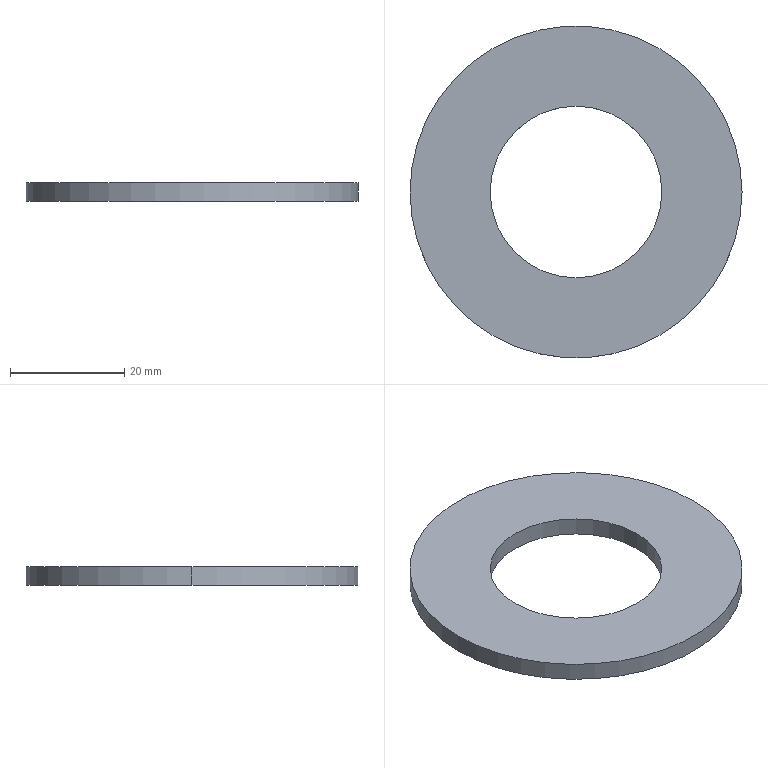Part | SolidWorks | features Extrusion 1 | 1 solid | 6 faces | box 58 x 58 x 3.2 mm | volume 6193 mm3 | cylinder 4 | plane 2 | commonest cylinder face diameters 30 x2 58 x2
STEP:
#1=CARTESIAN_POINT('',(-15.,0.,3.2));
#2=VERTEX_POINT('',#1);
#3=CARTESIAN_POINT('',(15.,0.,3.2));
#4=VERTEX_POINT('',#3);
#5=CARTESIAN_POINT('',(0.,0.,3.2));
#6=DIRECTION('',(0.,0.,1.));
#7=DIRECTION('',(1.,0.,0.));
#8=AXIS2_PLACEMENT_3D('',#5,#6,#7);
#9=CIRCLE('',#8,15.);
#10=EDGE_CURVE('',#2,#4,#9,.T.);
#11=ORIENTED_EDGE('',*,*,#10,.T.);
#12=CARTESIAN_POINT('',(15.,0.,0.));
#13=VERTEX_POINT('',#12);
#14=CARTESIAN_POINT('',(15.,0.,3.2));
#15=DIRECTION('',(0.,0.,-1.));
#16=VECTOR('',#15,1000.);
#17=LINE('',#14,#16);
#18=EDGE_CURVE('',#4,#13,#17,.T.);
#19=ORIENTED_EDGE('',*,*,#18,.T.);
#20=CARTESIAN_POINT('',(-15.,0.,0.));
#21=VERTEX_POINT('',#20);
#22=CARTESIAN_POINT('',(0.,0.,0.));
#23=DIRECTION('',(0.,0.,1.));
#24=DIRECTION('',(1.,0.,0.));
#25=AXIS2_PLACEMENT_3D('',#22,#23,#24);
#26=CIRCLE('',#25,15.);
#27=EDGE_CURVE('',#21,#13,#26,.T.);
#28=ORIENTED_EDGE('',*,*,#27,.F.);
#29=CARTESIAN_POINT('',(-15.,0.,3.2));
#30=DIRECTION('',(0.,0.,-1.));
#31=VECTOR('',#30,1000.);
#32=LINE('',#29,#31);
#33=EDGE_CURVE('',#2,#21,#32,.T.);
#34=ORIENTED_EDGE('',*,*,#33,.F.);
#35=EDGE_LOOP('',(#11,#19,#28,#34));
#36=FACE_OUTER_BOUND('',#35,.T.);
#37=CARTESIAN_POINT('',(0.,0.,3.2));
#38=DIRECTION('',(0.,0.,-1.));
#39=DIRECTION('',(-1.,0.,0.));
#40=AXIS2_PLACEMENT_3D('',#37,#38,#39);
#41=CYLINDRICAL_SURFACE('',#40,15.);
#42=ADVANCED_FACE('',(#36),#41,.F.);
#43=CARTESIAN_POINT('',(29.,0.,3.2));
#44=VERTEX_POINT('',#43);
#45=CARTESIAN_POINT('',(-29.,0.,3.2));
#46=VERTEX_POINT('',#45);
#47=CARTESIAN_POINT('',(0.,0.,3.2));
#48=DIRECTION('',(0.,0.,1.));
#49=DIRECTION('',(1.,0.,0.));
#50=AXIS2_PLACEMENT_3D('',#47,#48,#49);
#51=CIRCLE('',#50,29.);
#52=EDGE_CURVE('',#44,#46,#51,.T.);
#53=ORIENTED_EDGE('',*,*,#52,.F.);
#54=CARTESIAN_POINT('',(29.,0.,0.));
#55=VERTEX_POINT('',#54);
#56=CARTESIAN_POINT('',(29.,0.,3.2));
#57=DIRECTION('',(0.,0.,-1.));
#58=VECTOR('',#57,1000.);
#59=LINE('',#56,#58);
#60=EDGE_CURVE('',#44,#55,#59,.T.);
#61=ORIENTED_EDGE('',*,*,#60,.T.);
#62=CARTESIAN_POINT('',(-29.,0.,0.));
#63=VERTEX_POINT('',#62);
#64=CARTESIAN_POINT('',(0.,0.,0.));
#65=DIRECTION('',(0.,0.,1.));
#66=DIRECTION('',(1.,0.,0.));
#67=AXIS2_PLACEMENT_3D('',#64,#65,#66);
#68=CIRCLE('',#67,29.);
#69=EDGE_CURVE('',#55,#63,#68,.T.);
#70=ORIENTED_EDGE('',*,*,#69,.T.);
#71=CARTESIAN_POINT('',(-29.,0.,3.2));
#72=DIRECTION('',(0.,0.,-1.));
#73=VECTOR('',#72,1000.);
#74=LINE('',#71,#73);
#75=EDGE_CURVE('',#46,#63,#74,.T.);
#76=ORIENTED_EDGE('',*,*,#75,.F.);
#77=EDGE_LOOP('',(#53,#61,#70,#76));
#78=FACE_OUTER_BOUND('',#77,.T.);
#79=CARTESIAN_POINT('',(0.,0.,3.2));
#80=DIRECTION('',(0.,0.,-1.));
#81=DIRECTION('',(-1.,0.,0.));
#82=AXIS2_PLACEMENT_3D('',#79,#80,#81);
#83=CYLINDRICAL_SURFACE('',#82,29.);
#84=ADVANCED_FACE('',(#78),#83,.T.);
#85=CARTESIAN_POINT('',(0.,0.,3.2));
#86=DIRECTION('',(0.,0.,1.));
#87=DIRECTION('',(1.,0.,0.));
#88=AXIS2_PLACEMENT_3D('',#85,#86,#87);
#89=CIRCLE('',#88,29.);
#90=EDGE_CURVE('',#46,#44,#89,.T.);
#91=ORIENTED_EDGE('',*,*,#90,.T.);
#92=ORIENTED_EDGE('',*,*,#52,.T.);
#93=EDGE_LOOP('',(#91,#92));
#94=FACE_OUTER_BOUND('',#93,.T.);
#95=ORIENTED_EDGE('',*,*,#10,.F.);
#96=CARTESIAN_POINT('',(0.,0.,3.2));
#97=DIRECTION('',(0.,0.,1.));
#98=DIRECTION('',(1.,0.,0.));
#99=AXIS2_PLACEMENT_3D('',#96,#97,#98);
#100=CIRCLE('',#99,15.);
#101=EDGE_CURVE('',#4,#2,#100,.T.);
#102=ORIENTED_EDGE('',*,*,#101,.F.);
#103=EDGE_LOOP('',(#95,#102));
#104=FACE_BOUND('',#103,.T.);
#105=CARTESIAN_POINT('',(0.,0.,3.2));
#106=DIRECTION('',(0.,0.,1.));
#107=DIRECTION('',(1.,0.,0.));
#108=AXIS2_PLACEMENT_3D('',#105,#106,#107);
#109=PLANE('',#108);
#110=ADVANCED_FACE('',(#94,#104),#109,.T.);
#111=CARTESIAN_POINT('',(0.,0.,0.));
#112=DIRECTION('',(0.,0.,1.));
#113=DIRECTION('',(1.,0.,0.));
#114=AXIS2_PLACEMENT_3D('',#111,#112,#113);
#115=CIRCLE('',#114,29.);
#116=EDGE_CURVE('',#63,#55,#115,.T.);
#117=ORIENTED_EDGE('',*,*,#116,.F.);
#118=ORIENTED_EDGE('',*,*,#69,.F.);
#119=EDGE_LOOP('',(#117,#118));
#120=FACE_OUTER_BOUND('',#119,.T.);
#121=ORIENTED_EDGE('',*,*,#27,.T.);
#122=CARTESIAN_POINT('',(0.,0.,0.));
#123=DIRECTION('',(0.,0.,1.));
#124=DIRECTION('',(1.,0.,0.));
#125=AXIS2_PLACEMENT_3D('',#122,#123,#124);
#126=CIRCLE('',#125,15.);
#127=EDGE_CURVE('',#13,#21,#126,.T.);
#128=ORIENTED_EDGE('',*,*,#127,.T.);
#129=EDGE_LOOP('',(#121,#128));
#130=FACE_BOUND('',#129,.T.);
#131=CARTESIAN_POINT('',(0.,0.,0.));
#132=DIRECTION('',(0.,0.,1.));
#133=DIRECTION('',(1.,0.,0.));
#134=AXIS2_PLACEMENT_3D('',#131,#132,#133);
#135=PLANE('',#134);
#136=ADVANCED_FACE('',(#120,#130),#135,.F.);
#137=ORIENTED_EDGE('',*,*,#60,.F.);
#138=ORIENTED_EDGE('',*,*,#90,.F.);
#139=ORIENTED_EDGE('',*,*,#75,.T.);
#140=ORIENTED_EDGE('',*,*,#116,.T.);
#141=EDGE_LOOP('',(#137,#138,#139,#140));
#142=FACE_OUTER_BOUND('',#141,.T.);
#143=CARTESIAN_POINT('',(0.,0.,3.2));
#144=DIRECTION('',(0.,0.,-1.));
#145=DIRECTION('',(-1.,0.,0.));
#146=AXIS2_PLACEMENT_3D('',#143,#144,#145);
#147=CYLINDRICAL_SURFACE('',#146,29.);
#148=ADVANCED_FACE('',(#142),#147,.T.);
#149=ORIENTED_EDGE('',*,*,#18,.F.);
#150=ORIENTED_EDGE('',*,*,#101,.T.);
#151=ORIENTED_EDGE('',*,*,#33,.T.);
#152=ORIENTED_EDGE('',*,*,#127,.F.);
#153=EDGE_LOOP('',(#149,#150,#151,#152));
#154=FACE_OUTER_BOUND('',#153,.T.);
#155=CARTESIAN_POINT('',(0.,0.,3.2));
#156=DIRECTION('',(0.,0.,-1.));
#157=DIRECTION('',(-1.,0.,0.));
#158=AXIS2_PLACEMENT_3D('',#155,#156,#157);
#159=CYLINDRICAL_SURFACE('',#158,15.);
#160=ADVANCED_FACE('',(#154),#159,.F.);
#161=CLOSED_SHELL('',(#42,#84,#110,#136,#148,#160));
#162=MANIFOLD_SOLID_BREP('',#161);
#163=CARTESIAN_POINT('',(0.,0.,0.));
#164=DIRECTION('',(0.,0.,1.));
#165=DIRECTION('',(1.,0.,0.));
#166=AXIS2_PLACEMENT_3D('',#163,#164,#165);
#167=(LENGTH_UNIT()NAMED_UNIT(*)SI_UNIT(.MILLI.,.METRE.));
#168=UNCERTAINTY_MEASURE_WITH_UNIT(LENGTH_MEASURE(0.00001),#167,'','');
#169=(NAMED_UNIT(*)PLANE_ANGLE_UNIT()SI_UNIT($,.RADIAN.));
#170=(NAMED_UNIT(*)SI_UNIT($,.STERADIAN.)SOLID_ANGLE_UNIT());
#171=(GEOMETRIC_REPRESENTATION_CONTEXT(3)GLOBAL_UNCERTAINTY_ASSIGNED_CONTEXT((#168))GLOBAL_UNIT_ASSIGNED_CONTEXT((#167,#169,#170))REPRESENTATION_CONTEXT('',''));
#172=ADVANCED_BREP_SHAPE_REPRESENTATION('',(#162,#166),#171);